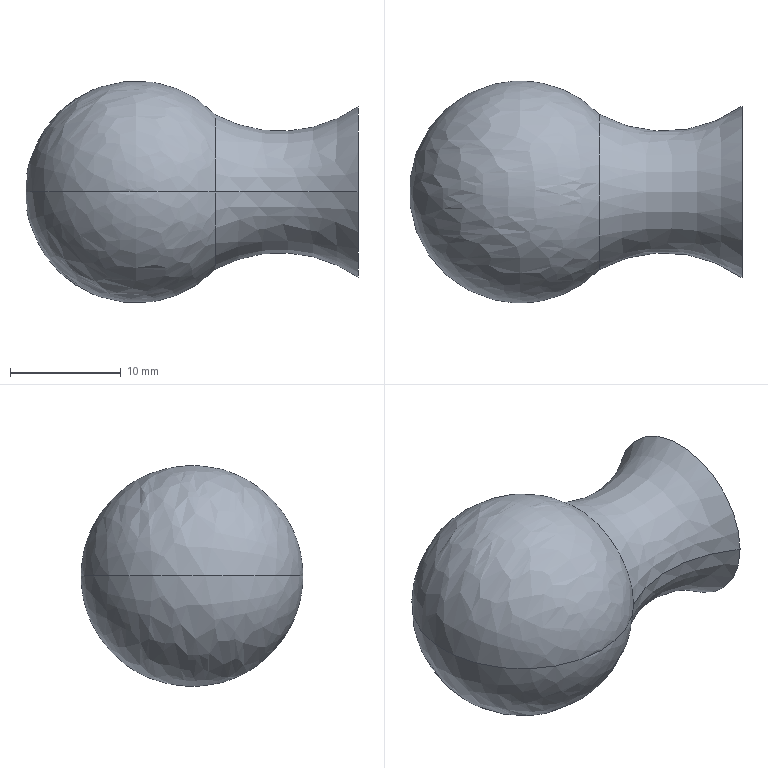Part | STEP file | Chrome small handle | 1 solid | 8 faces | volume 5297 mm3 | spline 4 | cylinder 2 | plane 2 | commonest cylinder face diameters 4.2 x2